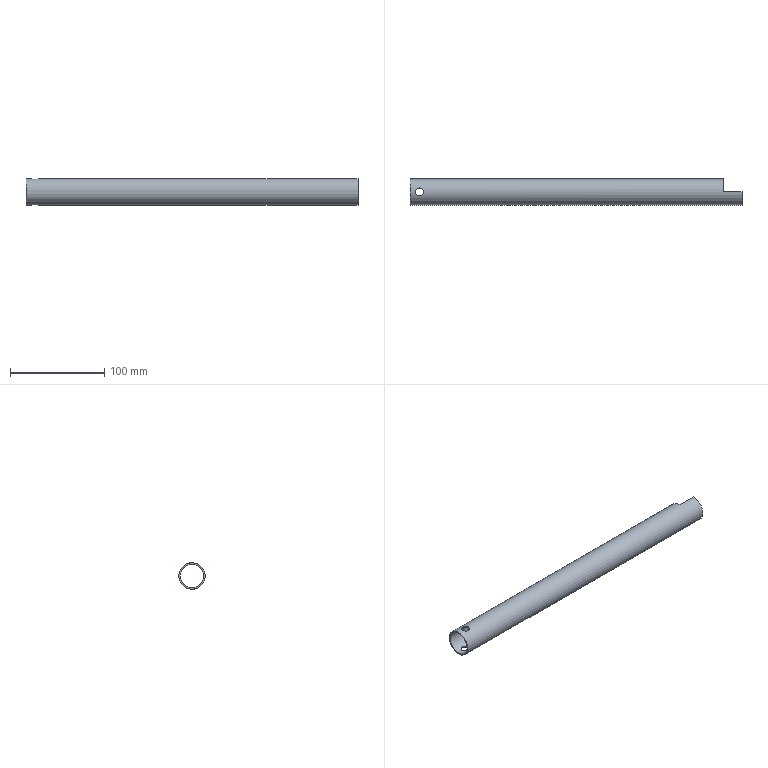Part | STEP file | GAS SHOCK 608W | 1 solid | 9 faces | box 353 x 28 x 28 mm | volume 42661 mm3 | plane 5 | cylinder 4 | commonest cylinder face diameters 8.5 x2 25 x1 28 x1
STEP:
#1=CARTESIAN_POINT('',(353.,0.,12.5));
#2=VERTEX_POINT('',#1);
#3=CARTESIAN_POINT('',(353.,0.,14.));
#4=VERTEX_POINT('',#3);
#5=CARTESIAN_POINT('',(353.,0.,-20.));
#6=DIRECTION('',(0.,0.,1.));
#7=VECTOR('',#6,1000.);
#8=LINE('',#5,#7);
#9=EDGE_CURVE('',#2,#4,#8,.T.);
#10=ORIENTED_EDGE('',*,*,#9,.T.);
#11=CARTESIAN_POINT('',(353.,0.,-14.));
#12=VERTEX_POINT('',#11);
#13=CARTESIAN_POINT('',(353.,0.,0.));
#14=DIRECTION('',(1.,0.,0.));
#15=DIRECTION('',(0.,0.,-1.));
#16=AXIS2_PLACEMENT_3D('',#13,#14,#15);
#17=CIRCLE('',#16,14.);
#18=EDGE_CURVE('',#4,#12,#17,.T.);
#19=ORIENTED_EDGE('',*,*,#18,.T.);
#20=CARTESIAN_POINT('',(353.,0.,-12.5));
#21=VERTEX_POINT('',#20);
#22=CARTESIAN_POINT('',(353.,0.,-20.));
#23=DIRECTION('',(0.,0.,1.));
#24=VECTOR('',#23,1000.);
#25=LINE('',#22,#24);
#26=EDGE_CURVE('',#12,#21,#25,.T.);
#27=ORIENTED_EDGE('',*,*,#26,.T.);
#28=CARTESIAN_POINT('',(353.,0.,0.));
#29=DIRECTION('',(1.,0.,0.));
#30=DIRECTION('',(0.,0.,-1.));
#31=AXIS2_PLACEMENT_3D('',#28,#29,#30);
#32=CIRCLE('',#31,12.5);
#33=EDGE_CURVE('',#2,#21,#32,.T.);
#34=ORIENTED_EDGE('',*,*,#33,.F.);
#35=EDGE_LOOP('',(#10,#19,#27,#34));
#36=FACE_OUTER_BOUND('',#35,.T.);
#37=CARTESIAN_POINT('',(353.,0.,0.));
#38=DIRECTION('',(1.,0.,0.));
#39=DIRECTION('',(0.,0.,-1.));
#40=AXIS2_PLACEMENT_3D('',#37,#38,#39);
#41=PLANE('',#40);
#42=ADVANCED_FACE('',(#36),#41,.T.);
#43=CARTESIAN_POINT('',(0.,0.,-14.));
#44=VERTEX_POINT('',#43);
#45=CARTESIAN_POINT('',(0.,0.,0.));
#46=DIRECTION('',(1.,0.,0.));
#47=DIRECTION('',(0.,0.,-1.));
#48=AXIS2_PLACEMENT_3D('',#45,#46,#47);
#49=CIRCLE('',#48,14.);
#50=EDGE_CURVE('',#44,#44,#49,.T.);
#51=ORIENTED_EDGE('',*,*,#50,.F.);
#52=EDGE_LOOP('',(#51));
#53=FACE_OUTER_BOUND('',#52,.T.);
#54=CARTESIAN_POINT('',(0.,0.,-12.5));
#55=VERTEX_POINT('',#54);
#56=CARTESIAN_POINT('',(0.,0.,0.));
#57=DIRECTION('',(1.,0.,0.));
#58=DIRECTION('',(0.,0.,-1.));
#59=AXIS2_PLACEMENT_3D('',#56,#57,#58);
#60=CIRCLE('',#59,12.5);
#61=EDGE_CURVE('',#55,#55,#60,.T.);
#62=ORIENTED_EDGE('',*,*,#61,.T.);
#63=EDGE_LOOP('',(#62));
#64=FACE_BOUND('',#63,.T.);
#65=CARTESIAN_POINT('',(0.,0.,0.));
#66=DIRECTION('',(1.,0.,0.));
#67=DIRECTION('',(0.,0.,-1.));
#68=AXIS2_PLACEMENT_3D('',#65,#66,#67);
#69=PLANE('',#68);
#70=ADVANCED_FACE('',(#53,#64),#69,.F.);
#71=CARTESIAN_POINT('',(14.25,0.,14.));
#72=VERTEX_POINT('',#71);
#73=CARTESIAN_POINT('',(14.25,0.,14.));
#74=CARTESIAN_POINT('',(14.25,-0.2826,14.));
#75=CARTESIAN_POINT('',(14.222,-0.5601,13.991));
#76=CARTESIAN_POINT('',(14.113,-1.106,13.959));
#77=CARTESIAN_POINT('',(14.031,-1.376,13.935));
#78=CARTESIAN_POINT('',(13.817,-1.89,13.874));
#79=CARTESIAN_POINT('',(13.686,-2.134,13.838));
#80=CARTESIAN_POINT('',(13.377,-2.595,13.759));
#81=CARTESIAN_POINT('',(13.199,-2.811,13.716));
#82=CARTESIAN_POINT('',(12.81,-3.201,13.631));
#83=CARTESIAN_POINT('',(12.597,-3.376,13.588));
#84=CARTESIAN_POINT('',(12.133,-3.687,13.507));
#85=CARTESIAN_POINT('',(11.888,-3.818,13.47));
#86=CARTESIAN_POINT('',(11.378,-4.03,13.408));
#87=CARTESIAN_POINT('',(11.108,-4.113,13.382));
#88=CARTESIAN_POINT('',(10.559,-4.222,13.348));
#89=CARTESIAN_POINT('',(10.282,-4.25,13.339));
#90=CARTESIAN_POINT('',(9.724,-4.25,13.339));
#91=CARTESIAN_POINT('',(9.44,-4.222,13.348));
#92=CARTESIAN_POINT('',(8.894,-4.113,13.382));
#93=CARTESIAN_POINT('',(8.628,-4.032,13.407));
#94=CARTESIAN_POINT('',(8.111,-3.818,13.47));
#95=CARTESIAN_POINT('',(7.866,-3.686,13.507));
#96=CARTESIAN_POINT('',(7.407,-3.379,13.587));
#97=CARTESIAN_POINT('',(7.191,-3.201,13.631));
#98=CARTESIAN_POINT('',(6.799,-2.809,13.717));
#99=CARTESIAN_POINT('',(6.624,-2.596,13.759));
#100=CARTESIAN_POINT('',(6.316,-2.137,13.838));
#101=CARTESIAN_POINT('',(6.182,-1.888,13.874));
#102=CARTESIAN_POINT('',(5.969,-1.376,13.935));
#103=CARTESIAN_POINT('',(5.888,-1.111,13.959));
#104=CARTESIAN_POINT('',(5.778,-0.5622,13.991));
#105=CARTESIAN_POINT('',(5.75,-0.2802,14.));
#106=CARTESIAN_POINT('',(5.75,0.2766,14.));
#107=CARTESIAN_POINT('',(5.777,0.556,13.992));
#108=CARTESIAN_POINT('',(5.887,1.108,13.959));
#109=CARTESIAN_POINT('',(5.969,1.374,13.935));
#110=CARTESIAN_POINT('',(6.181,1.886,13.875));
#111=CARTESIAN_POINT('',(6.315,2.135,13.838));
#112=CARTESIAN_POINT('',(6.623,2.595,13.759));
#113=CARTESIAN_POINT('',(6.798,2.808,13.717));
#114=CARTESIAN_POINT('',(7.19,3.2,13.631));
#115=CARTESIAN_POINT('',(7.406,3.378,13.587));
#116=CARTESIAN_POINT('',(7.864,3.684,13.507));
#117=CARTESIAN_POINT('',(8.108,3.816,13.47));
#118=CARTESIAN_POINT('',(8.626,4.031,13.407));
#119=CARTESIAN_POINT('',(8.891,4.112,13.383));
#120=CARTESIAN_POINT('',(9.436,4.222,13.348));
#121=CARTESIAN_POINT('',(9.719,4.25,13.339));
#122=CARTESIAN_POINT('',(10.279,4.25,13.339));
#123=CARTESIAN_POINT('',(10.556,4.223,13.348));
#124=CARTESIAN_POINT('',(11.104,4.114,13.382));
#125=CARTESIAN_POINT('',(11.375,4.031,13.408));
#126=CARTESIAN_POINT('',(11.887,3.818,13.47));
#127=CARTESIAN_POINT('',(12.131,3.688,13.507));
#128=CARTESIAN_POINT('',(12.596,3.377,13.588));
#129=CARTESIAN_POINT('',(12.809,3.201,13.631));
#130=CARTESIAN_POINT('',(13.199,2.812,13.716));
#131=CARTESIAN_POINT('',(13.377,2.595,13.759));
#132=CARTESIAN_POINT('',(13.686,2.135,13.838));
#133=CARTESIAN_POINT('',(13.816,1.891,13.874));
#134=CARTESIAN_POINT('',(14.03,1.379,13.934));
#135=CARTESIAN_POINT('',(14.113,1.107,13.959));
#136=CARTESIAN_POINT('',(14.222,0.5605,13.991));
#137=CARTESIAN_POINT('',(14.25,0.2826,14.));
#138=CARTESIAN_POINT('',(14.25,0.,14.));
#139=B_SPLINE_CURVE_WITH_KNOTS('',3,(#73,#74,#75,#76,#77,#78,#79,#80,#81,#82,#83,#84,#85,#86,#87,#88,#89,#90,#91,#92,#93,#94,#95,#96,#97,#98,#99,#100,#101,#102,#103,#104,#105,#106,#107,#108,#109,#110,#111,#112,#113,#114,#115,#116,#117,#118,#119,#120,#121,#122,#123,#124,#125,#126,#127,#128,#129,#130,#131,#132,#133,#134,#135,#136,#137,#138),.UNSPECIFIED.,.T.,.F.,(4,2,2,2,2,2,2,2,2,2,2,2,2,2,2,2,2,2,2,2,2,2,2,2,2,2,2,2,2,2,2,2,4),(0.,0.0008353,0.001671,0.002506,0.003341,0.004177,0.005012,0.005847,0.006682,0.007518,0.008353,0.009188,0.01002,0.01086,0.01169,0.01253,0.01336,0.0142,0.01504,0.01587,0.01671,0.01754,0.01838,0.01921,0.02005,0.02088,0.02172,0.02255,0.02339,0.02422,0.02506,0.02589,0.02673),.UNSPECIFIED.);
#140=EDGE_CURVE('',#72,#72,#139,.T.);
#141=ORIENTED_EDGE('',*,*,#140,.T.);
#142=EDGE_LOOP('',(#141));
#143=FACE_BOUND('',#142,.T.);
#144=CARTESIAN_POINT('',(14.25,0.,-14.));
#145=VERTEX_POINT('',#144);
#146=CARTESIAN_POINT('',(14.25,0.,-14.));
#147=CARTESIAN_POINT('',(14.25,0.2826,-14.));
#148=CARTESIAN_POINT('',(14.222,0.5601,-13.991));
#149=CARTESIAN_POINT('',(14.113,1.106,-13.959));
#150=CARTESIAN_POINT('',(14.031,1.376,-13.935));
#151=CARTESIAN_POINT('',(13.817,1.89,-13.874));
#152=CARTESIAN_POINT('',(13.686,2.134,-13.838));
#153=CARTESIAN_POINT('',(13.377,2.595,-13.759));
#154=CARTESIAN_POINT('',(13.199,2.811,-13.716));
#155=CARTESIAN_POINT('',(12.81,3.201,-13.631));
#156=CARTESIAN_POINT('',(12.597,3.376,-13.588));
#157=CARTESIAN_POINT('',(12.133,3.687,-13.507));
#158=CARTESIAN_POINT('',(11.888,3.818,-13.47));
#159=CARTESIAN_POINT('',(11.378,4.03,-13.408));
#160=CARTESIAN_POINT('',(11.108,4.113,-13.382));
#161=CARTESIAN_POINT('',(10.559,4.222,-13.348));
#162=CARTESIAN_POINT('',(10.282,4.25,-13.339));
#163=CARTESIAN_POINT('',(9.724,4.25,-13.339));
#164=CARTESIAN_POINT('',(9.44,4.222,-13.348));
#165=CARTESIAN_POINT('',(8.894,4.113,-13.382));
#166=CARTESIAN_POINT('',(8.628,4.032,-13.407));
#167=CARTESIAN_POINT('',(8.111,3.818,-13.47));
#168=CARTESIAN_POINT('',(7.866,3.686,-13.507));
#169=CARTESIAN_POINT('',(7.407,3.379,-13.587));
#170=CARTESIAN_POINT('',(7.191,3.201,-13.631));
#171=CARTESIAN_POINT('',(6.799,2.809,-13.717));
#172=CARTESIAN_POINT('',(6.624,2.596,-13.759));
#173=CARTESIAN_POINT('',(6.316,2.137,-13.838));
#174=CARTESIAN_POINT('',(6.182,1.888,-13.874));
#175=CARTESIAN_POINT('',(5.969,1.376,-13.935));
#176=CARTESIAN_POINT('',(5.888,1.111,-13.959));
#177=CARTESIAN_POINT('',(5.778,0.5622,-13.991));
#178=CARTESIAN_POINT('',(5.75,0.2802,-14.));
#179=CARTESIAN_POINT('',(5.75,-0.2766,-14.));
#180=CARTESIAN_POINT('',(5.777,-0.556,-13.992));
#181=CARTESIAN_POINT('',(5.887,-1.108,-13.959));
#182=CARTESIAN_POINT('',(5.969,-1.374,-13.935));
#183=CARTESIAN_POINT('',(6.181,-1.886,-13.875));
#184=CARTESIAN_POINT('',(6.315,-2.135,-13.838));
#185=CARTESIAN_POINT('',(6.623,-2.595,-13.759));
#186=CARTESIAN_POINT('',(6.798,-2.808,-13.717));
#187=CARTESIAN_POINT('',(7.19,-3.2,-13.631));
#188=CARTESIAN_POINT('',(7.406,-3.378,-13.587));
#189=CARTESIAN_POINT('',(7.864,-3.684,-13.507));
#190=CARTESIAN_POINT('',(8.108,-3.816,-13.47));
#191=CARTESIAN_POINT('',(8.626,-4.031,-13.407));
#192=CARTESIAN_POINT('',(8.891,-4.112,-13.383));
#193=CARTESIAN_POINT('',(9.436,-4.222,-13.348));
#194=CARTESIAN_POINT('',(9.719,-4.25,-13.339));
#195=CARTESIAN_POINT('',(10.279,-4.25,-13.339));
#196=CARTESIAN_POINT('',(10.556,-4.223,-13.348));
#197=CARTESIAN_POINT('',(11.104,-4.114,-13.382));
#198=CARTESIAN_POINT('',(11.375,-4.031,-13.408));
#199=CARTESIAN_POINT('',(11.887,-3.818,-13.47));
#200=CARTESIAN_POINT('',(12.131,-3.688,-13.507));
#201=CARTESIAN_POINT('',(12.596,-3.377,-13.588));
#202=CARTESIAN_POINT('',(12.809,-3.201,-13.631));
#203=CARTESIAN_POINT('',(13.199,-2.812,-13.716));
#204=CARTESIAN_POINT('',(13.377,-2.595,-13.759));
#205=CARTESIAN_POINT('',(13.686,-2.135,-13.838));
#206=CARTESIAN_POINT('',(13.816,-1.891,-13.874));
#207=CARTESIAN_POINT('',(14.03,-1.379,-13.934));
#208=CARTESIAN_POINT('',(14.113,-1.107,-13.959));
#209=CARTESIAN_POINT('',(14.222,-0.5605,-13.991));
#210=CARTESIAN_POINT('',(14.25,-0.2826,-14.));
#211=CARTESIAN_POINT('',(14.25,0.,-14.));
#212=B_SPLINE_CURVE_WITH_KNOTS('',3,(#146,#147,#148,#149,#150,#151,#152,#153,#154,#155,#156,#157,#158,#159,#160,#161,#162,#163,#164,#165,#166,#167,#168,#169,#170,#171,#172,#173,#174,#175,#176,#177,#178,#179,#180,#181,#182,#183,#184,#185,#186,#187,#188,#189,#190,#191,#192,#193,#194,#195,#196,#197,#198,#199,#200,#201,#202,#203,#204,#205,#206,#207,#208,#209,#210,#211),.UNSPECIFIED.,.T.,.F.,(4,2,2,2,2,2,2,2,2,2,2,2,2,2,2,2,2,2,2,2,2,2,2,2,2,2,2,2,2,2,2,2,4),(0.,0.0008353,0.001671,0.002506,0.003341,0.004177,0.005012,0.005847,0.006682,0.007518,0.008353,0.009188,0.01002,0.01086,0.01169,0.01253,0.01336,0.0142,0.01504,0.01587,0.01671,0.01754,0.01838,0.01921,0.02005,0.02088,0.02172,0.02255,0.02339,0.02422,0.02506,0.02589,0.02673),.UNSPECIFIED.);
#213=EDGE_CURVE('',#145,#145,#212,.T.);
#214=ORIENTED_EDGE('',*,*,#213,.T.);
#215=EDGE_LOOP('',(#214));
#216=FACE_BOUND('',#215,.T.);
#217=ORIENTED_EDGE('',*,*,#18,.F.);
#218=CARTESIAN_POINT('',(333.,0.,14.));
#219=VERTEX_POINT('',#218);
#220=CARTESIAN_POINT('',(353.,0.,14.));
#221=DIRECTION('',(-1.,0.,0.));
#222=VECTOR('',#221,1000.);
#223=LINE('',#220,#222);
#224=EDGE_CURVE('',#4,#219,#223,.T.);
#225=ORIENTED_EDGE('',*,*,#224,.T.);
#226=CARTESIAN_POINT('',(333.,0.,-14.));
#227=VERTEX_POINT('',#226);
#228=CARTESIAN_POINT('',(333.,0.,0.));
#229=DIRECTION('',(-1.,0.,0.));
#230=DIRECTION('',(0.,0.,1.));
#231=AXIS2_PLACEMENT_3D('',#228,#229,#230);
#232=CIRCLE('',#231,14.);
#233=EDGE_CURVE('',#219,#227,#232,.T.);
#234=ORIENTED_EDGE('',*,*,#233,.T.);
#235=CARTESIAN_POINT('',(353.,0.,-14.));
#236=DIRECTION('',(1.,0.,0.));
#237=VECTOR('',#236,1000.);
#238=LINE('',#235,#237);
#239=EDGE_CURVE('',#227,#12,#238,.T.);
#240=ORIENTED_EDGE('',*,*,#239,.T.);
#241=EDGE_LOOP('',(#217,#225,#234,#240));
#242=FACE_OUTER_BOUND('',#241,.T.);
#243=ORIENTED_EDGE('',*,*,#50,.T.);
#244=EDGE_LOOP('',(#243));
#245=FACE_OUTER_BOUND('',#244,.T.);
#246=CARTESIAN_POINT('',(353.,0.,0.));
#247=DIRECTION('',(-1.,0.,0.));
#248=DIRECTION('',(0.,0.,1.));
#249=AXIS2_PLACEMENT_3D('',#246,#247,#248);
#250=CYLINDRICAL_SURFACE('',#249,14.);
#251=ADVANCED_FACE('',(#143,#216,#242,#245),#250,.T.);
#252=CARTESIAN_POINT('',(333.,0.,12.5));
#253=VERTEX_POINT('',#252);
#254=CARTESIAN_POINT('',(353.,0.,12.5));
#255=DIRECTION('',(-1.,0.,0.));
#256=VECTOR('',#255,1000.);
#257=LINE('',#254,#256);
#258=EDGE_CURVE('',#2,#253,#257,.T.);
#259=ORIENTED_EDGE('',*,*,#258,.F.);
#260=ORIENTED_EDGE('',*,*,#33,.T.);
#261=CARTESIAN_POINT('',(333.,0.,-12.5));
#262=VERTEX_POINT('',#261);
#263=CARTESIAN_POINT('',(353.,0.,-12.5));
#264=DIRECTION('',(1.,0.,0.));
#265=VECTOR('',#264,1000.);
#266=LINE('',#263,#265);
#267=EDGE_CURVE('',#262,#21,#266,.T.);
#268=ORIENTED_EDGE('',*,*,#267,.F.);
#269=CARTESIAN_POINT('',(333.,0.,0.));
#270=DIRECTION('',(-1.,0.,0.));
#271=DIRECTION('',(0.,0.,1.));
#272=AXIS2_PLACEMENT_3D('',#269,#270,#271);
#273=CIRCLE('',#272,12.5);
#274=EDGE_CURVE('',#253,#262,#273,.T.);
#275=ORIENTED_EDGE('',*,*,#274,.F.);
#276=EDGE_LOOP('',(#259,#260,#268,#275));
#277=FACE_OUTER_BOUND('',#276,.T.);
#278=CARTESIAN_POINT('',(14.25,0.,12.5));
#279=VERTEX_POINT('',#278);
#280=CARTESIAN_POINT('',(14.25,0.,12.5));
#281=CARTESIAN_POINT('',(14.25,-0.283,12.5));
#282=CARTESIAN_POINT('',(14.222,-0.561,12.49));
#283=CARTESIAN_POINT('',(14.113,-1.107,12.454));
#284=CARTESIAN_POINT('',(14.03,-1.378,12.426));
#285=CARTESIAN_POINT('',(13.816,-1.892,12.359));
#286=CARTESIAN_POINT('',(13.685,-2.135,12.318));
#287=CARTESIAN_POINT('',(13.377,-2.596,12.23));
#288=CARTESIAN_POINT('',(13.199,-2.812,12.181));
#289=CARTESIAN_POINT('',(12.81,-3.201,12.085));
#290=CARTESIAN_POINT('',(12.597,-3.376,12.037));
#291=CARTESIAN_POINT('',(12.133,-3.686,11.945));
#292=CARTESIAN_POINT('',(11.89,-3.817,11.904));
#293=CARTESIAN_POINT('',(11.379,-4.029,11.833));
#294=CARTESIAN_POINT('',(11.109,-4.112,11.804));
#295=CARTESIAN_POINT('',(10.56,-4.222,11.765));
#296=CARTESIAN_POINT('',(10.283,-4.25,11.755));
#297=CARTESIAN_POINT('',(9.723,-4.25,11.755));
#298=CARTESIAN_POINT('',(9.439,-4.222,11.766));
#299=CARTESIAN_POINT('',(8.893,-4.113,11.804));
#300=CARTESIAN_POINT('',(8.627,-4.032,11.833));
#301=CARTESIAN_POINT('',(8.109,-3.817,11.904));
#302=CARTESIAN_POINT('',(7.864,-3.685,11.946));
#303=CARTESIAN_POINT('',(7.406,-3.378,12.036));
#304=CARTESIAN_POINT('',(7.19,-3.2,12.085));
#305=CARTESIAN_POINT('',(6.799,-2.809,12.182));
#306=CARTESIAN_POINT('',(6.625,-2.597,12.229));
#307=CARTESIAN_POINT('',(6.317,-2.138,12.318));
#308=CARTESIAN_POINT('',(6.183,-1.889,12.359));
#309=CARTESIAN_POINT('',(5.97,-1.378,12.427));
#310=CARTESIAN_POINT('',(5.889,-1.113,12.453));
#311=CARTESIAN_POINT('',(5.778,-0.5622,12.49));
#312=CARTESIAN_POINT('',(5.75,-0.2805,12.5));
#313=CARTESIAN_POINT('',(5.75,0.2771,12.5));
#314=CARTESIAN_POINT('',(5.777,0.5581,12.491));
#315=CARTESIAN_POINT('',(5.888,1.11,12.454));
#316=CARTESIAN_POINT('',(5.969,1.375,12.427));
#317=CARTESIAN_POINT('',(6.183,1.888,12.359));
#318=CARTESIAN_POINT('',(6.316,2.137,12.318));
#319=CARTESIAN_POINT('',(6.624,2.596,12.23));
#320=CARTESIAN_POINT('',(6.798,2.809,12.182));
#321=CARTESIAN_POINT('',(7.387,3.398,12.036));
#322=CARTESIAN_POINT('',(7.851,3.709,11.939));
#323=CARTESIAN_POINT('',(8.625,4.031,11.833));
#324=CARTESIAN_POINT('',(8.89,4.112,11.804));
#325=CARTESIAN_POINT('',(9.436,4.222,11.766));
#326=CARTESIAN_POINT('',(9.72,4.25,11.755));
#327=CARTESIAN_POINT('',(10.28,4.25,11.755));
#328=CARTESIAN_POINT('',(10.557,4.223,11.765));
#329=CARTESIAN_POINT('',(11.107,4.113,11.804));
#330=CARTESIAN_POINT('',(11.377,4.03,11.833));
#331=CARTESIAN_POINT('',(11.889,3.817,11.903));
#332=CARTESIAN_POINT('',(12.135,3.685,11.946));
#333=CARTESIAN_POINT('',(12.597,3.376,12.037));
#334=CARTESIAN_POINT('',(12.81,3.201,12.085));
#335=CARTESIAN_POINT('',(13.199,2.811,12.181));
#336=CARTESIAN_POINT('',(13.378,2.594,12.23));
#337=CARTESIAN_POINT('',(13.685,2.135,12.319));
#338=CARTESIAN_POINT('',(13.816,1.892,12.359));
#339=CARTESIAN_POINT('',(14.03,1.378,12.427));
#340=CARTESIAN_POINT('',(14.113,1.107,12.454));
#341=CARTESIAN_POINT('',(14.222,0.5611,12.49));
#342=CARTESIAN_POINT('',(14.25,0.283,12.5));
#343=CARTESIAN_POINT('',(14.25,0.,12.5));
#344=B_SPLINE_CURVE_WITH_KNOTS('',3,(#280,#281,#282,#283,#284,#285,#286,#287,#288,#289,#290,#291,#292,#293,#294,#295,#296,#297,#298,#299,#300,#301,#302,#303,#304,#305,#306,#307,#308,#309,#310,#311,#312,#313,#314,#315,#316,#317,#318,#319,#320,#321,#322,#323,#324,#325,#326,#327,#328,#329,#330,#331,#332,#333,#334,#335,#336,#337,#338,#339,#340,#341,#342,#343),.UNSPECIFIED.,.T.,.F.,(4,2,2,2,2,2,2,2,2,2,2,2,2,2,2,2,2,2,2,2,2,2,2,2,2,2,2,2,2,2,2,4),(0.,0.0008366,0.001673,0.00251,0.003347,0.004183,0.00502,0.005857,0.006693,0.00753,0.008366,0.009203,0.01004,0.01088,0.01171,0.01255,0.01339,0.01422,0.01506,0.0159,0.01673,0.01841,0.01924,0.02008,0.02092,0.02175,0.02259,0.02343,0.02426,0.0251,0.02594,0.02677),.UNSPECIFIED.);
#345=EDGE_CURVE('',#279,#279,#344,.T.);
#346=ORIENTED_EDGE('',*,*,#345,.F.);
#347=EDGE_LOOP('',(#346));
#348=FACE_BOUND('',#347,.T.);
#349=CARTESIAN_POINT('',(14.25,0.,-12.5));
#350=VERTEX_POINT('',#349);
#351=CARTESIAN_POINT('',(14.25,0.,-12.5));
#352=CARTESIAN_POINT('',(14.25,0.283,-12.5));
#353=CARTESIAN_POINT('',(14.222,0.561,-12.49));
#354=CARTESIAN_POINT('',(14.113,1.107,-12.454));
#355=CARTESIAN_POINT('',(14.03,1.378,-12.426));
#356=CARTESIAN_POINT('',(13.816,1.892,-12.359));
#357=CARTESIAN_POINT('',(13.685,2.135,-12.318));
#358=CARTESIAN_POINT('',(13.377,2.596,-12.23));
#359=CARTESIAN_POINT('',(13.199,2.812,-12.181));
#360=CARTESIAN_POINT('',(12.81,3.201,-12.085));
#361=CARTESIAN_POINT('',(12.597,3.376,-12.037));
#362=CARTESIAN_POINT('',(12.133,3.686,-11.945));
#363=CARTESIAN_POINT('',(11.89,3.817,-11.904));
#364=CARTESIAN_POINT('',(11.379,4.029,-11.833));
#365=CARTESIAN_POINT('',(11.109,4.112,-11.804));
#366=CARTESIAN_POINT('',(10.56,4.222,-11.765));
#367=CARTESIAN_POINT('',(10.283,4.25,-11.755));
#368=CARTESIAN_POINT('',(9.723,4.25,-11.755));
#369=CARTESIAN_POINT('',(9.439,4.222,-11.766));
#370=CARTESIAN_POINT('',(8.893,4.113,-11.804));
#371=CARTESIAN_POINT('',(8.627,4.032,-11.833));
#372=CARTESIAN_POINT('',(8.109,3.817,-11.904));
#373=CARTESIAN_POINT('',(7.864,3.685,-11.946));
#374=CARTESIAN_POINT('',(7.406,3.378,-12.036));
#375=CARTESIAN_POINT('',(7.19,3.2,-12.085));
#376=CARTESIAN_POINT('',(6.799,2.809,-12.182));
#377=CARTESIAN_POINT('',(6.625,2.597,-12.229));
#378=CARTESIAN_POINT('',(6.317,2.138,-12.318));
#379=CARTESIAN_POINT('',(6.183,1.889,-12.359));
#380=CARTESIAN_POINT('',(5.97,1.378,-12.427));
#381=CARTESIAN_POINT('',(5.889,1.113,-12.453));
#382=CARTESIAN_POINT('',(5.778,0.5622,-12.49));
#383=CARTESIAN_POINT('',(5.75,0.2805,-12.5));
#384=CARTESIAN_POINT('',(5.75,-0.2771,-12.5));
#385=CARTESIAN_POINT('',(5.777,-0.5581,-12.491));
#386=CARTESIAN_POINT('',(5.888,-1.11,-12.454));
#387=CARTESIAN_POINT('',(5.969,-1.375,-12.427));
#388=CARTESIAN_POINT('',(6.183,-1.888,-12.359));
#389=CARTESIAN_POINT('',(6.316,-2.137,-12.318));
#390=CARTESIAN_POINT('',(6.624,-2.596,-12.23));
#391=CARTESIAN_POINT('',(6.798,-2.809,-12.182));
#392=CARTESIAN_POINT('',(7.387,-3.398,-12.036));
#393=CARTESIAN_POINT('',(7.851,-3.709,-11.939));
#394=CARTESIAN_POINT('',(8.625,-4.031,-11.833));
#395=CARTESIAN_POINT('',(8.89,-4.112,-11.804));
#396=CARTESIAN_POINT('',(9.436,-4.222,-11.766));
#397=CARTESIAN_POINT('',(9.72,-4.25,-11.755));
#398=CARTESIAN_POINT('',(10.28,-4.25,-11.755));
#399=CARTESIAN_POINT('',(10.557,-4.223,-11.765));
#400=CARTESIAN_POINT('',(11.107,-4.113,-11.804));
#401=CARTESIAN_POINT('',(11.377,-4.03,-11.833));
#402=CARTESIAN_POINT('',(11.889,-3.817,-11.903));
#403=CARTESIAN_POINT('',(12.135,-3.685,-11.946));
#404=CARTESIAN_POINT('',(12.597,-3.376,-12.037));
#405=CARTESIAN_POINT('',(12.81,-3.201,-12.085));
#406=CARTESIAN_POINT('',(13.199,-2.811,-12.181));
#407=CARTESIAN_POINT('',(13.378,-2.594,-12.23));
#408=CARTESIAN_POINT('',(13.685,-2.135,-12.319));
#409=CARTESIAN_POINT('',(13.816,-1.892,-12.359));
#410=CARTESIAN_POINT('',(14.03,-1.378,-12.427));
#411=CARTESIAN_POINT('',(14.113,-1.107,-12.454));
#412=CARTESIAN_POINT('',(14.222,-0.5611,-12.49));
#413=CARTESIAN_POINT('',(14.25,-0.283,-12.5));
#414=CARTESIAN_POINT('',(14.25,0.,-12.5));
#415=B_SPLINE_CURVE_WITH_KNOTS('',3,(#351,#352,#353,#354,#355,#356,#357,#358,#359,#360,#361,#362,#363,#364,#365,#366,#367,#368,#369,#370,#371,#372,#373,#374,#375,#376,#377,#378,#379,#380,#381,#382,#383,#384,#385,#386,#387,#388,#389,#390,#391,#392,#393,#394,#395,#396,#397,#398,#399,#400,#401,#402,#403,#404,#405,#406,#407,#408,#409,#410,#411,#412,#413,#414),.UNSPECIFIED.,.T.,.F.,(4,2,2,2,2,2,2,2,2,2,2,2,2,2,2,2,2,2,2,2,2,2,2,2,2,2,2,2,2,2,2,4),(0.,0.0008366,0.001673,0.00251,0.003347,0.004183,0.00502,0.005857,0.006693,0.00753,0.008366,0.009203,0.01004,0.01088,0.01171,0.01255,0.01339,0.01422,0.01506,0.0159,0.01673,0.01841,0.01924,0.02008,0.02092,0.02175,0.02259,0.02343,0.02426,0.0251,0.02594,0.02677),.UNSPECIFIED.);
#416=EDGE_CURVE('',#350,#350,#415,.T.);
#417=ORIENTED_EDGE('',*,*,#416,.F.);
#418=EDGE_LOOP('',(#417));
#419=FACE_BOUND('',#418,.T.);
#420=ORIENTED_EDGE('',*,*,#61,.F.);
#421=EDGE_LOOP('',(#420));
#422=FACE_OUTER_BOUND('',#421,.T.);
#423=CARTESIAN_POINT('',(353.,0.,0.));
#424=DIRECTION('',(-1.,0.,0.));
#425=DIRECTION('',(0.,0.,1.));
#426=AXIS2_PLACEMENT_3D('',#423,#424,#425);
#427=CYLINDRICAL_SURFACE('',#426,12.5);
#428=ADVANCED_FACE('',(#277,#348,#419,#422),#427,.F.);
#429=ORIENTED_EDGE('',*,*,#416,.T.);
#430=EDGE_LOOP('',(#429));
#431=FACE_OUTER_BOUND('',#430,.T.);
#432=ORIENTED_EDGE('',*,*,#213,.F.);
#433=EDGE_LOOP('',(#432));
#434=FACE_OUTER_BOUND('',#433,.T.);
#435=CARTESIAN_POINT('',(10.,0.,-20.));
#436=DIRECTION('',(0.,0.,1.));
#437=DIRECTION('',(1.,0.,0.));
#438=AXIS2_PLACEMENT_3D('',#435,#436,#437);
#439=CYLINDRICAL_SURFACE('',#438,4.25);
#440=ADVANCED_FACE('',(#431,#434),#439,.F.);
#441=ORIENTED_EDGE('',*,*,#345,.T.);
#442=EDGE_LOOP('',(#441));
#443=FACE_OUTER_BOUND('',#442,.T.);
#444=ORIENTED_EDGE('',*,*,#140,.F.);
#445=EDGE_LOOP('',(#444));
#446=FACE_OUTER_BOUND('',#445,.T.);
#447=CARTESIAN_POINT('',(10.,0.,-20.));
#448=DIRECTION('',(0.,0.,1.));
#449=DIRECTION('',(1.,0.,0.));
#450=AXIS2_PLACEMENT_3D('',#447,#448,#449);
#451=CYLINDRICAL_SURFACE('',#450,4.25);
#452=ADVANCED_FACE('',(#443,#446),#451,.F.);
#453=ORIENTED_EDGE('',*,*,#9,.F.);
#454=ORIENTED_EDGE('',*,*,#258,.T.);
#455=CARTESIAN_POINT('',(333.,0.,-20.));
#456=DIRECTION('',(0.,0.,1.));
#457=VECTOR('',#456,1000.);
#458=LINE('',#455,#457);
#459=EDGE_CURVE('',#253,#219,#458,.T.);
#460=ORIENTED_EDGE('',*,*,#459,.T.);
#461=ORIENTED_EDGE('',*,*,#224,.F.);
#462=EDGE_LOOP('',(#453,#454,#460,#461));
#463=FACE_OUTER_BOUND('',#462,.T.);
#464=CARTESIAN_POINT('',(353.,0.,-20.));
#465=DIRECTION('',(0.,-1.,0.));
#466=DIRECTION('',(1.,0.,0.));
#467=AXIS2_PLACEMENT_3D('',#464,#465,#466);
#468=PLANE('',#467);
#469=ADVANCED_FACE('',(#463),#468,.F.);
#470=CARTESIAN_POINT('',(333.,0.,-20.));
#471=DIRECTION('',(0.,0.,1.));
#472=VECTOR('',#471,1000.);
#473=LINE('',#470,#472);
#474=EDGE_CURVE('',#227,#262,#473,.T.);
#475=ORIENTED_EDGE('',*,*,#474,.T.);
#476=ORIENTED_EDGE('',*,*,#267,.T.);
#477=ORIENTED_EDGE('',*,*,#26,.F.);
#478=ORIENTED_EDGE('',*,*,#239,.F.);
#479=EDGE_LOOP('',(#475,#476,#477,#478));
#480=FACE_OUTER_BOUND('',#479,.T.);
#481=CARTESIAN_POINT('',(353.,0.,-20.));
#482=DIRECTION('',(0.,-1.,0.));
#483=DIRECTION('',(1.,0.,0.));
#484=AXIS2_PLACEMENT_3D('',#481,#482,#483);
#485=PLANE('',#484);
#486=ADVANCED_FACE('',(#480),#485,.F.);
#487=ORIENTED_EDGE('',*,*,#459,.F.);
#488=ORIENTED_EDGE('',*,*,#274,.T.);
#489=ORIENTED_EDGE('',*,*,#474,.F.);
#490=ORIENTED_EDGE('',*,*,#233,.F.);
#491=EDGE_LOOP('',(#487,#488,#489,#490));
#492=FACE_OUTER_BOUND('',#491,.T.);
#493=CARTESIAN_POINT('',(333.,14.,-20.));
#494=DIRECTION('',(-1.,0.,0.));
#495=DIRECTION('',(0.,0.,1.));
#496=AXIS2_PLACEMENT_3D('',#493,#494,#495);
#497=PLANE('',#496);
#498=ADVANCED_FACE('',(#492),#497,.F.);
#499=CLOSED_SHELL('',(#42,#70,#251,#428,#440,#452,#469,#486,#498));
#500=MANIFOLD_SOLID_BREP('',#499);
#501=CARTESIAN_POINT('',(0.,0.,0.));
#502=DIRECTION('',(0.,0.,1.));
#503=DIRECTION('',(1.,0.,0.));
#504=AXIS2_PLACEMENT_3D('',#501,#502,#503);
#505=(LENGTH_UNIT()NAMED_UNIT(*)SI_UNIT(.MILLI.,.METRE.));
#506=UNCERTAINTY_MEASURE_WITH_UNIT(LENGTH_MEASURE(0.00001),#505,'','');
#507=(NAMED_UNIT(*)PLANE_ANGLE_UNIT()SI_UNIT($,.RADIAN.));
#508=(NAMED_UNIT(*)SI_UNIT($,.STERADIAN.)SOLID_ANGLE_UNIT());
#509=(GEOMETRIC_REPRESENTATION_CONTEXT(3)GLOBAL_UNCERTAINTY_ASSIGNED_CONTEXT((#506))GLOBAL_UNIT_ASSIGNED_CONTEXT((#505,#507,#508))REPRESENTATION_CONTEXT('',''));
#510=ADVANCED_BREP_SHAPE_REPRESENTATION('',(#500,#504),#509);